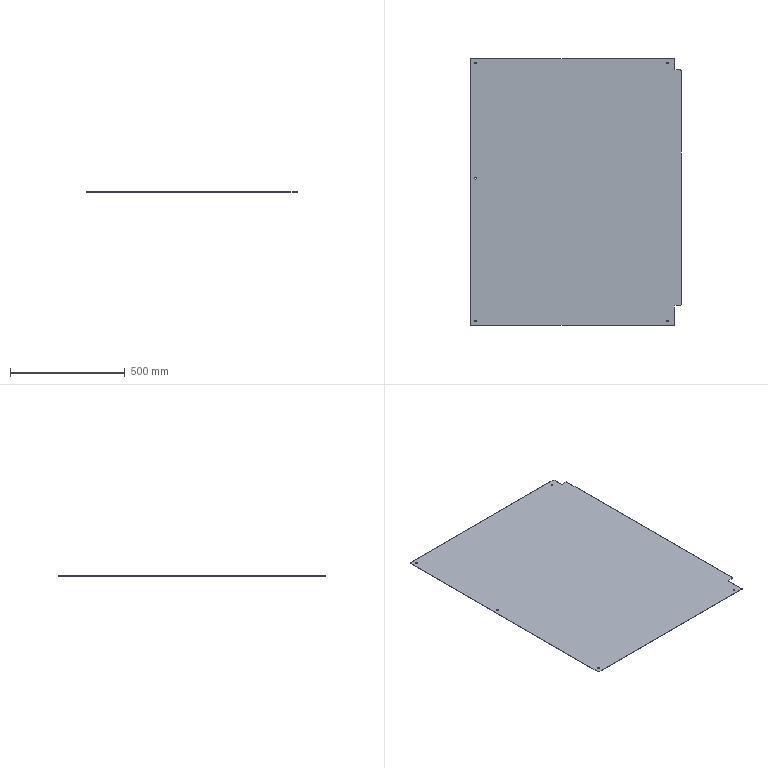Part | SolidWorks | features Fillet 1, FlatPattern 1, HoleWzd 1, ICE 1, SMBaseFlange 1, SheetMetal 1 | 1 solid | 28 faces | box 915 x 1162 x 1.2 mm | volume 1270668 mm3 | cylinder 18 | plane 10 | commonest cylinder face diameters 7 x10 6 x8
STEP:
#1=CARTESIAN_POINT('',(16.5,-20.,0.));
#2=VERTEX_POINT('',#1);
#3=CARTESIAN_POINT('',(23.5,-20.,0.));
#4=VERTEX_POINT('',#3);
#5=CARTESIAN_POINT('',(20.,-20.,0.));
#6=DIRECTION('',(0.,0.,1.));
#7=DIRECTION('',(1.,0.,0.));
#8=AXIS2_PLACEMENT_3D('',#5,#6,#7);
#9=CIRCLE('',#8,3.5);
#10=EDGE_CURVE('',#2,#4,#9,.T.);
#11=ORIENTED_EDGE('',*,*,#10,.F.);
#12=CARTESIAN_POINT('',(16.5,-20.,1.2));
#13=VERTEX_POINT('',#12);
#14=CARTESIAN_POINT('',(16.5,-20.,1.2));
#15=DIRECTION('',(0.,0.,1.));
#16=VECTOR('',#15,1000.);
#17=LINE('',#14,#16);
#18=EDGE_CURVE('',#2,#13,#17,.T.);
#19=ORIENTED_EDGE('',*,*,#18,.T.);
#20=CARTESIAN_POINT('',(23.5,-20.,1.2));
#21=VERTEX_POINT('',#20);
#22=CARTESIAN_POINT('',(20.,-20.,1.2));
#23=DIRECTION('',(0.,0.,1.));
#24=DIRECTION('',(1.,0.,0.));
#25=AXIS2_PLACEMENT_3D('',#22,#23,#24);
#26=CIRCLE('',#25,3.5);
#27=EDGE_CURVE('',#13,#21,#26,.T.);
#28=ORIENTED_EDGE('',*,*,#27,.T.);
#29=CARTESIAN_POINT('',(23.5,-20.,1.2));
#30=DIRECTION('',(0.,0.,1.));
#31=VECTOR('',#30,1000.);
#32=LINE('',#29,#31);
#33=EDGE_CURVE('',#4,#21,#32,.T.);
#34=ORIENTED_EDGE('',*,*,#33,.F.);
#35=EDGE_LOOP('',(#11,#19,#28,#34));
#36=FACE_OUTER_BOUND('',#35,.T.);
#37=CARTESIAN_POINT('',(20.,-20.,1.2));
#38=DIRECTION('',(0.,0.,1.));
#39=DIRECTION('',(1.,0.,0.));
#40=AXIS2_PLACEMENT_3D('',#37,#38,#39);
#41=CYLINDRICAL_SURFACE('',#40,3.5);
#42=ADVANCED_FACE('',(#36),#41,.F.);
#43=CARTESIAN_POINT('',(851.5,-20.,0.));
#44=VERTEX_POINT('',#43);
#45=CARTESIAN_POINT('',(858.5,-20.,0.));
#46=VERTEX_POINT('',#45);
#47=CARTESIAN_POINT('',(855.,-20.,0.));
#48=DIRECTION('',(0.,0.,1.));
#49=DIRECTION('',(1.,0.,0.));
#50=AXIS2_PLACEMENT_3D('',#47,#48,#49);
#51=CIRCLE('',#50,3.5);
#52=EDGE_CURVE('',#44,#46,#51,.T.);
#53=ORIENTED_EDGE('',*,*,#52,.F.);
#54=CARTESIAN_POINT('',(851.5,-20.,1.2));
#55=VERTEX_POINT('',#54);
#56=CARTESIAN_POINT('',(851.5,-20.,1.2));
#57=DIRECTION('',(0.,0.,1.));
#58=VECTOR('',#57,1000.);
#59=LINE('',#56,#58);
#60=EDGE_CURVE('',#44,#55,#59,.T.);
#61=ORIENTED_EDGE('',*,*,#60,.T.);
#62=CARTESIAN_POINT('',(858.5,-20.,1.2));
#63=VERTEX_POINT('',#62);
#64=CARTESIAN_POINT('',(855.,-20.,1.2));
#65=DIRECTION('',(0.,0.,1.));
#66=DIRECTION('',(1.,0.,0.));
#67=AXIS2_PLACEMENT_3D('',#64,#65,#66);
#68=CIRCLE('',#67,3.5);
#69=EDGE_CURVE('',#55,#63,#68,.T.);
#70=ORIENTED_EDGE('',*,*,#69,.T.);
#71=CARTESIAN_POINT('',(858.5,-20.,1.2));
#72=DIRECTION('',(0.,0.,1.));
#73=VECTOR('',#72,1000.);
#74=LINE('',#71,#73);
#75=EDGE_CURVE('',#46,#63,#74,.T.);
#76=ORIENTED_EDGE('',*,*,#75,.F.);
#77=EDGE_LOOP('',(#53,#61,#70,#76));
#78=FACE_OUTER_BOUND('',#77,.T.);
#79=CARTESIAN_POINT('',(855.,-20.,1.2));
#80=DIRECTION('',(0.,0.,1.));
#81=DIRECTION('',(1.,0.,0.));
#82=AXIS2_PLACEMENT_3D('',#79,#80,#81);
#83=CYLINDRICAL_SURFACE('',#82,3.5);
#84=ADVANCED_FACE('',(#78),#83,.F.);
#85=CARTESIAN_POINT('',(16.5,-1142.,0.));
#86=VERTEX_POINT('',#85);
#87=CARTESIAN_POINT('',(23.5,-1142.,0.));
#88=VERTEX_POINT('',#87);
#89=CARTESIAN_POINT('',(20.,-1142.,0.));
#90=DIRECTION('',(0.,0.,1.));
#91=DIRECTION('',(1.,0.,0.));
#92=AXIS2_PLACEMENT_3D('',#89,#90,#91);
#93=CIRCLE('',#92,3.5);
#94=EDGE_CURVE('',#86,#88,#93,.T.);
#95=ORIENTED_EDGE('',*,*,#94,.F.);
#96=CARTESIAN_POINT('',(16.5,-1142.,1.2));
#97=VERTEX_POINT('',#96);
#98=CARTESIAN_POINT('',(16.5,-1142.,1.2));
#99=DIRECTION('',(0.,0.,1.));
#100=VECTOR('',#99,1000.);
#101=LINE('',#98,#100);
#102=EDGE_CURVE('',#86,#97,#101,.T.);
#103=ORIENTED_EDGE('',*,*,#102,.T.);
#104=CARTESIAN_POINT('',(23.5,-1142.,1.2));
#105=VERTEX_POINT('',#104);
#106=CARTESIAN_POINT('',(20.,-1142.,1.2));
#107=DIRECTION('',(0.,0.,1.));
#108=DIRECTION('',(1.,0.,0.));
#109=AXIS2_PLACEMENT_3D('',#106,#107,#108);
#110=CIRCLE('',#109,3.5);
#111=EDGE_CURVE('',#97,#105,#110,.T.);
#112=ORIENTED_EDGE('',*,*,#111,.T.);
#113=CARTESIAN_POINT('',(23.5,-1142.,1.2));
#114=DIRECTION('',(0.,0.,1.));
#115=VECTOR('',#114,1000.);
#116=LINE('',#113,#115);
#117=EDGE_CURVE('',#88,#105,#116,.T.);
#118=ORIENTED_EDGE('',*,*,#117,.F.);
#119=EDGE_LOOP('',(#95,#103,#112,#118));
#120=FACE_OUTER_BOUND('',#119,.T.);
#121=CARTESIAN_POINT('',(20.,-1142.,1.2));
#122=DIRECTION('',(0.,0.,1.));
#123=DIRECTION('',(1.,0.,0.));
#124=AXIS2_PLACEMENT_3D('',#121,#122,#123);
#125=CYLINDRICAL_SURFACE('',#124,3.5);
#126=ADVANCED_FACE('',(#120),#125,.F.);
#127=CARTESIAN_POINT('',(851.5,-1142.,0.));
#128=VERTEX_POINT('',#127);
#129=CARTESIAN_POINT('',(858.5,-1142.,0.));
#130=VERTEX_POINT('',#129);
#131=CARTESIAN_POINT('',(855.,-1142.,0.));
#132=DIRECTION('',(0.,0.,1.));
#133=DIRECTION('',(1.,0.,0.));
#134=AXIS2_PLACEMENT_3D('',#131,#132,#133);
#135=CIRCLE('',#134,3.5);
#136=EDGE_CURVE('',#128,#130,#135,.T.);
#137=ORIENTED_EDGE('',*,*,#136,.F.);
#138=CARTESIAN_POINT('',(851.5,-1142.,1.2));
#139=VERTEX_POINT('',#138);
#140=CARTESIAN_POINT('',(851.5,-1142.,1.2));
#141=DIRECTION('',(0.,0.,1.));
#142=VECTOR('',#141,1000.);
#143=LINE('',#140,#142);
#144=EDGE_CURVE('',#128,#139,#143,.T.);
#145=ORIENTED_EDGE('',*,*,#144,.T.);
#146=CARTESIAN_POINT('',(858.5,-1142.,1.2));
#147=VERTEX_POINT('',#146);
#148=CARTESIAN_POINT('',(855.,-1142.,1.2));
#149=DIRECTION('',(0.,0.,1.));
#150=DIRECTION('',(1.,0.,0.));
#151=AXIS2_PLACEMENT_3D('',#148,#149,#150);
#152=CIRCLE('',#151,3.5);
#153=EDGE_CURVE('',#139,#147,#152,.T.);
#154=ORIENTED_EDGE('',*,*,#153,.T.);
#155=CARTESIAN_POINT('',(858.5,-1142.,1.2));
#156=DIRECTION('',(0.,0.,1.));
#157=VECTOR('',#156,1000.);
#158=LINE('',#155,#157);
#159=EDGE_CURVE('',#130,#147,#158,.T.);
#160=ORIENTED_EDGE('',*,*,#159,.F.);
#161=EDGE_LOOP('',(#137,#145,#154,#160));
#162=FACE_OUTER_BOUND('',#161,.T.);
#163=CARTESIAN_POINT('',(855.,-1142.,1.2));
#164=DIRECTION('',(0.,0.,1.));
#165=DIRECTION('',(1.,0.,0.));
#166=AXIS2_PLACEMENT_3D('',#163,#164,#165);
#167=CYLINDRICAL_SURFACE('',#166,3.5);
#168=ADVANCED_FACE('',(#162),#167,.F.);
#169=CARTESIAN_POINT('',(16.5,-522.,0.));
#170=VERTEX_POINT('',#169);
#171=CARTESIAN_POINT('',(23.5,-522.,0.));
#172=VERTEX_POINT('',#171);
#173=CARTESIAN_POINT('',(20.,-522.,0.));
#174=DIRECTION('',(0.,0.,1.));
#175=DIRECTION('',(1.,0.,0.));
#176=AXIS2_PLACEMENT_3D('',#173,#174,#175);
#177=CIRCLE('',#176,3.5);
#178=EDGE_CURVE('',#170,#172,#177,.T.);
#179=ORIENTED_EDGE('',*,*,#178,.F.);
#180=CARTESIAN_POINT('',(16.5,-522.,1.2));
#181=VERTEX_POINT('',#180);
#182=CARTESIAN_POINT('',(16.5,-522.,1.2));
#183=DIRECTION('',(0.,0.,1.));
#184=VECTOR('',#183,1000.);
#185=LINE('',#182,#184);
#186=EDGE_CURVE('',#170,#181,#185,.T.);
#187=ORIENTED_EDGE('',*,*,#186,.T.);
#188=CARTESIAN_POINT('',(23.5,-522.,1.2));
#189=VERTEX_POINT('',#188);
#190=CARTESIAN_POINT('',(20.,-522.,1.2));
#191=DIRECTION('',(0.,0.,1.));
#192=DIRECTION('',(1.,0.,0.));
#193=AXIS2_PLACEMENT_3D('',#190,#191,#192);
#194=CIRCLE('',#193,3.5);
#195=EDGE_CURVE('',#181,#189,#194,.T.);
#196=ORIENTED_EDGE('',*,*,#195,.T.);
#197=CARTESIAN_POINT('',(23.5,-522.,1.2));
#198=DIRECTION('',(0.,0.,1.));
#199=VECTOR('',#198,1000.);
#200=LINE('',#197,#199);
#201=EDGE_CURVE('',#172,#189,#200,.T.);
#202=ORIENTED_EDGE('',*,*,#201,.F.);
#203=EDGE_LOOP('',(#179,#187,#196,#202));
#204=FACE_OUTER_BOUND('',#203,.T.);
#205=CARTESIAN_POINT('',(20.,-522.,1.2));
#206=DIRECTION('',(0.,0.,1.));
#207=DIRECTION('',(1.,0.,0.));
#208=AXIS2_PLACEMENT_3D('',#205,#206,#207);
#209=CYLINDRICAL_SURFACE('',#208,3.5);
#210=ADVANCED_FACE('',(#204),#209,.F.);
#211=CARTESIAN_POINT('',(0.,-1159.,0.));
#212=VERTEX_POINT('',#211);
#213=CARTESIAN_POINT('',(0.,-3.,0.));
#214=VERTEX_POINT('',#213);
#215=CARTESIAN_POINT('',(0.,0.,0.));
#216=DIRECTION('',(0.,1.,0.));
#217=VECTOR('',#216,1000.);
#218=LINE('',#215,#217);
#219=EDGE_CURVE('',#212,#214,#218,.T.);
#220=ORIENTED_EDGE('',*,*,#219,.F.);
#221=CARTESIAN_POINT('',(0.,-1159.,1.2));
#222=VERTEX_POINT('',#221);
#223=CARTESIAN_POINT('',(0.,-1159.,1.2));
#224=DIRECTION('',(0.,0.,1.));
#225=VECTOR('',#224,1000.);
#226=LINE('',#223,#225);
#227=EDGE_CURVE('',#212,#222,#226,.T.);
#228=ORIENTED_EDGE('',*,*,#227,.T.);
#229=CARTESIAN_POINT('',(0.,-3.,1.2));
#230=VERTEX_POINT('',#229);
#231=CARTESIAN_POINT('',(0.,0.,1.2));
#232=DIRECTION('',(0.,1.,0.));
#233=VECTOR('',#232,1000.);
#234=LINE('',#231,#233);
#235=EDGE_CURVE('',#222,#230,#234,.T.);
#236=ORIENTED_EDGE('',*,*,#235,.T.);
#237=CARTESIAN_POINT('',(0.,-3.,1.2));
#238=DIRECTION('',(0.,0.,-1.));
#239=VECTOR('',#238,1000.);
#240=LINE('',#237,#239);
#241=EDGE_CURVE('',#230,#214,#240,.T.);
#242=ORIENTED_EDGE('',*,*,#241,.T.);
#243=EDGE_LOOP('',(#220,#228,#236,#242));
#244=FACE_OUTER_BOUND('',#243,.T.);
#245=CARTESIAN_POINT('',(0.,0.,1.2));
#246=DIRECTION('',(-1.,0.,0.));
#247=DIRECTION('',(0.,0.,1.));
#248=AXIS2_PLACEMENT_3D('',#245,#246,#247);
#249=PLANE('',#248);
#250=ADVANCED_FACE('',(#244),#249,.T.);
#251=CARTESIAN_POINT('',(882.,-1162.,1.2));
#252=VERTEX_POINT('',#251);
#253=CARTESIAN_POINT('',(3.,-1162.,1.2));
#254=VERTEX_POINT('',#253);
#255=CARTESIAN_POINT('',(0.,-1162.,1.2));
#256=DIRECTION('',(-1.,0.,0.));
#257=VECTOR('',#256,1000.);
#258=LINE('',#255,#257);
#259=EDGE_CURVE('',#252,#254,#258,.T.);
#260=ORIENTED_EDGE('',*,*,#259,.T.);
#261=CARTESIAN_POINT('',(3.,-1162.,0.));
#262=VERTEX_POINT('',#261);
#263=CARTESIAN_POINT('',(3.,-1162.,1.2));
#264=DIRECTION('',(0.,0.,-1.));
#265=VECTOR('',#264,1000.);
#266=LINE('',#263,#265);
#267=EDGE_CURVE('',#254,#262,#266,.T.);
#268=ORIENTED_EDGE('',*,*,#267,.T.);
#269=CARTESIAN_POINT('',(882.,-1162.,0.));
#270=VERTEX_POINT('',#269);
#271=CARTESIAN_POINT('',(0.,-1162.,0.));
#272=DIRECTION('',(-1.,0.,0.));
#273=VECTOR('',#272,1000.);
#274=LINE('',#271,#273);
#275=EDGE_CURVE('',#270,#262,#274,.T.);
#276=ORIENTED_EDGE('',*,*,#275,.F.);
#277=CARTESIAN_POINT('',(882.,-1162.,1.2));
#278=DIRECTION('',(0.,0.,1.));
#279=VECTOR('',#278,1000.);
#280=LINE('',#277,#279);
#281=EDGE_CURVE('',#270,#252,#280,.T.);
#282=ORIENTED_EDGE('',*,*,#281,.T.);
#283=EDGE_LOOP('',(#260,#268,#276,#282));
#284=FACE_OUTER_BOUND('',#283,.T.);
#285=CARTESIAN_POINT('',(0.,-1162.,1.2));
#286=DIRECTION('',(0.,-1.,0.));
#287=DIRECTION('',(0.,0.,-1.));
#288=AXIS2_PLACEMENT_3D('',#285,#286,#287);
#289=PLANE('',#288);
#290=ADVANCED_FACE('',(#284),#289,.T.);
#291=CARTESIAN_POINT('',(915.,-53.,1.2));
#292=VERTEX_POINT('',#291);
#293=CARTESIAN_POINT('',(915.,-1071.,1.2));
#294=VERTEX_POINT('',#293);
#295=CARTESIAN_POINT('',(915.,0.,1.2));
#296=DIRECTION('',(0.,-1.,0.));
#297=VECTOR('',#296,1000.);
#298=LINE('',#295,#297);
#299=EDGE_CURVE('',#292,#294,#298,.T.);
#300=ORIENTED_EDGE('',*,*,#299,.T.);
#301=CARTESIAN_POINT('',(915.,-1071.,0.));
#302=VERTEX_POINT('',#301);
#303=CARTESIAN_POINT('',(915.,-1071.,0.));
#304=DIRECTION('',(0.,0.,-1.));
#305=VECTOR('',#304,1000.);
#306=LINE('',#303,#305);
#307=EDGE_CURVE('',#294,#302,#306,.T.);
#308=ORIENTED_EDGE('',*,*,#307,.T.);
#309=CARTESIAN_POINT('',(915.,-53.,0.));
#310=VERTEX_POINT('',#309);
#311=CARTESIAN_POINT('',(915.,0.,0.));
#312=DIRECTION('',(0.,-1.,0.));
#313=VECTOR('',#312,1000.);
#314=LINE('',#311,#313);
#315=EDGE_CURVE('',#310,#302,#314,.T.);
#316=ORIENTED_EDGE('',*,*,#315,.F.);
#317=CARTESIAN_POINT('',(915.,-53.,1.2));
#318=DIRECTION('',(0.,0.,1.));
#319=VECTOR('',#318,1000.);
#320=LINE('',#317,#319);
#321=EDGE_CURVE('',#310,#292,#320,.T.);
#322=ORIENTED_EDGE('',*,*,#321,.T.);
#323=EDGE_LOOP('',(#300,#308,#316,#322));
#324=FACE_OUTER_BOUND('',#323,.T.);
#325=CARTESIAN_POINT('',(915.,0.,1.2));
#326=DIRECTION('',(1.,0.,0.));
#327=DIRECTION('',(0.,0.,-1.));
#328=AXIS2_PLACEMENT_3D('',#325,#326,#327);
#329=PLANE('',#328);
#330=ADVANCED_FACE('',(#324),#329,.T.);
#331=CARTESIAN_POINT('',(3.,0.,1.2));
#332=VERTEX_POINT('',#331);
#333=CARTESIAN_POINT('',(882.,0.,1.2));
#334=VERTEX_POINT('',#333);
#335=CARTESIAN_POINT('',(0.,0.,1.2));
#336=DIRECTION('',(1.,0.,0.));
#337=VECTOR('',#336,1000.);
#338=LINE('',#335,#337);
#339=EDGE_CURVE('',#332,#334,#338,.T.);
#340=ORIENTED_EDGE('',*,*,#339,.T.);
#341=CARTESIAN_POINT('',(882.,0.,0.));
#342=VERTEX_POINT('',#341);
#343=CARTESIAN_POINT('',(882.,0.,0.));
#344=DIRECTION('',(0.,0.,-1.));
#345=VECTOR('',#344,1000.);
#346=LINE('',#343,#345);
#347=EDGE_CURVE('',#334,#342,#346,.T.);
#348=ORIENTED_EDGE('',*,*,#347,.T.);
#349=CARTESIAN_POINT('',(3.,0.,0.));
#350=VERTEX_POINT('',#349);
#351=CARTESIAN_POINT('',(0.,0.,0.));
#352=DIRECTION('',(1.,0.,0.));
#353=VECTOR('',#352,1000.);
#354=LINE('',#351,#353);
#355=EDGE_CURVE('',#350,#342,#354,.T.);
#356=ORIENTED_EDGE('',*,*,#355,.F.);
#357=CARTESIAN_POINT('',(3.,0.,1.2));
#358=DIRECTION('',(0.,0.,1.));
#359=VECTOR('',#358,1000.);
#360=LINE('',#357,#359);
#361=EDGE_CURVE('',#350,#332,#360,.T.);
#362=ORIENTED_EDGE('',*,*,#361,.T.);
#363=EDGE_LOOP('',(#340,#348,#356,#362));
#364=FACE_OUTER_BOUND('',#363,.T.);
#365=CARTESIAN_POINT('',(0.,0.,1.2));
#366=DIRECTION('',(0.,1.,0.));
#367=DIRECTION('',(0.,0.,1.));
#368=AXIS2_PLACEMENT_3D('',#365,#366,#367);
#369=PLANE('',#368);
#370=ADVANCED_FACE('',(#364),#369,.T.);
#371=CARTESIAN_POINT('',(20.,-20.,1.2));
#372=DIRECTION('',(0.,0.,1.));
#373=DIRECTION('',(1.,0.,0.));
#374=AXIS2_PLACEMENT_3D('',#371,#372,#373);
#375=CIRCLE('',#374,3.5);
#376=EDGE_CURVE('',#21,#13,#375,.T.);
#377=ORIENTED_EDGE('',*,*,#376,.F.);
#378=ORIENTED_EDGE('',*,*,#27,.F.);
#379=EDGE_LOOP('',(#377,#378));
#380=FACE_BOUND('',#379,.T.);
#381=CARTESIAN_POINT('',(855.,-20.,1.2));
#382=DIRECTION('',(0.,0.,1.));
#383=DIRECTION('',(1.,0.,0.));
#384=AXIS2_PLACEMENT_3D('',#381,#382,#383);
#385=CIRCLE('',#384,3.5);
#386=EDGE_CURVE('',#63,#55,#385,.T.);
#387=ORIENTED_EDGE('',*,*,#386,.F.);
#388=ORIENTED_EDGE('',*,*,#69,.F.);
#389=EDGE_LOOP('',(#387,#388));
#390=FACE_BOUND('',#389,.T.);
#391=CARTESIAN_POINT('',(20.,-1142.,1.2));
#392=DIRECTION('',(0.,0.,1.));
#393=DIRECTION('',(1.,0.,0.));
#394=AXIS2_PLACEMENT_3D('',#391,#392,#393);
#395=CIRCLE('',#394,3.5);
#396=EDGE_CURVE('',#105,#97,#395,.T.);
#397=ORIENTED_EDGE('',*,*,#396,.F.);
#398=ORIENTED_EDGE('',*,*,#111,.F.);
#399=EDGE_LOOP('',(#397,#398));
#400=FACE_BOUND('',#399,.T.);
#401=CARTESIAN_POINT('',(855.,-1142.,1.2));
#402=DIRECTION('',(0.,0.,1.));
#403=DIRECTION('',(1.,0.,0.));
#404=AXIS2_PLACEMENT_3D('',#401,#402,#403);
#405=CIRCLE('',#404,3.5);
#406=EDGE_CURVE('',#147,#139,#405,.T.);
#407=ORIENTED_EDGE('',*,*,#406,.F.);
#408=ORIENTED_EDGE('',*,*,#153,.F.);
#409=EDGE_LOOP('',(#407,#408));
#410=FACE_BOUND('',#409,.T.);
#411=CARTESIAN_POINT('',(20.,-522.,1.2));
#412=DIRECTION('',(0.,0.,1.));
#413=DIRECTION('',(1.,0.,0.));
#414=AXIS2_PLACEMENT_3D('',#411,#412,#413);
#415=CIRCLE('',#414,3.5);
#416=EDGE_CURVE('',#189,#181,#415,.T.);
#417=ORIENTED_EDGE('',*,*,#416,.F.);
#418=ORIENTED_EDGE('',*,*,#195,.F.);
#419=EDGE_LOOP('',(#417,#418));
#420=FACE_BOUND('',#419,.T.);
#421=ORIENTED_EDGE('',*,*,#235,.F.);
#422=CARTESIAN_POINT('',(3.,-1159.,1.2));
#423=DIRECTION('',(0.,0.,1.));
#424=DIRECTION('',(1.,0.,0.));
#425=AXIS2_PLACEMENT_3D('',#422,#423,#424);
#426=CIRCLE('',#425,3.);
#427=EDGE_CURVE('',#222,#254,#426,.T.);
#428=ORIENTED_EDGE('',*,*,#427,.T.);
#429=ORIENTED_EDGE('',*,*,#259,.F.);
#430=CARTESIAN_POINT('',(885.,-1159.,1.2));
#431=VERTEX_POINT('',#430);
#432=CARTESIAN_POINT('',(882.,-1159.,1.2));
#433=DIRECTION('',(0.,0.,1.));
#434=DIRECTION('',(1.,0.,0.));
#435=AXIS2_PLACEMENT_3D('',#432,#433,#434);
#436=CIRCLE('',#435,3.);
#437=EDGE_CURVE('',#252,#431,#436,.T.);
#438=ORIENTED_EDGE('',*,*,#437,.T.);
#439=CARTESIAN_POINT('',(885.,-1077.,1.2));
#440=VERTEX_POINT('',#439);
#441=CARTESIAN_POINT('',(885.,-1162.,1.2));
#442=DIRECTION('',(0.,-1.,0.));
#443=VECTOR('',#442,1000.);
#444=LINE('',#441,#443);
#445=EDGE_CURVE('',#440,#431,#444,.T.);
#446=ORIENTED_EDGE('',*,*,#445,.F.);
#447=CARTESIAN_POINT('',(888.,-1074.,1.2));
#448=VERTEX_POINT('',#447);
#449=CARTESIAN_POINT('',(888.,-1077.,1.2));
#450=DIRECTION('',(0.,0.,-1.));
#451=DIRECTION('',(1.,0.,0.));
#452=AXIS2_PLACEMENT_3D('',#449,#450,#451);
#453=CIRCLE('',#452,3.);
#454=EDGE_CURVE('',#440,#448,#453,.T.);
#455=ORIENTED_EDGE('',*,*,#454,.T.);
#456=CARTESIAN_POINT('',(912.,-1074.,1.2));
#457=VERTEX_POINT('',#456);
#458=CARTESIAN_POINT('',(915.,-1074.,1.2));
#459=DIRECTION('',(-1.,0.,0.));
#460=VECTOR('',#459,1000.);
#461=LINE('',#458,#460);
#462=EDGE_CURVE('',#457,#448,#461,.T.);
#463=ORIENTED_EDGE('',*,*,#462,.F.);
#464=CARTESIAN_POINT('',(912.,-1071.,1.2));
#465=DIRECTION('',(0.,0.,1.));
#466=DIRECTION('',(1.,0.,0.));
#467=AXIS2_PLACEMENT_3D('',#464,#465,#466);
#468=CIRCLE('',#467,3.);
#469=EDGE_CURVE('',#457,#294,#468,.T.);
#470=ORIENTED_EDGE('',*,*,#469,.T.);
#471=ORIENTED_EDGE('',*,*,#299,.F.);
#472=CARTESIAN_POINT('',(912.,-50.,1.2));
#473=VERTEX_POINT('',#472);
#474=CARTESIAN_POINT('',(912.,-53.,1.2));
#475=DIRECTION('',(0.,0.,1.));
#476=DIRECTION('',(1.,0.,0.));
#477=AXIS2_PLACEMENT_3D('',#474,#475,#476);
#478=CIRCLE('',#477,3.);
#479=EDGE_CURVE('',#292,#473,#478,.T.);
#480=ORIENTED_EDGE('',*,*,#479,.T.);
#481=CARTESIAN_POINT('',(888.,-50.,1.2));
#482=VERTEX_POINT('',#481);
#483=CARTESIAN_POINT('',(915.,-50.,1.2));
#484=DIRECTION('',(1.,0.,0.));
#485=VECTOR('',#484,1000.);
#486=LINE('',#483,#485);
#487=EDGE_CURVE('',#482,#473,#486,.T.);
#488=ORIENTED_EDGE('',*,*,#487,.F.);
#489=CARTESIAN_POINT('',(885.,-47.,1.2));
#490=VERTEX_POINT('',#489);
#491=CARTESIAN_POINT('',(888.,-47.,1.2));
#492=DIRECTION('',(0.,0.,-1.));
#493=DIRECTION('',(1.,0.,0.));
#494=AXIS2_PLACEMENT_3D('',#491,#492,#493);
#495=CIRCLE('',#494,3.);
#496=EDGE_CURVE('',#482,#490,#495,.T.);
#497=ORIENTED_EDGE('',*,*,#496,.T.);
#498=CARTESIAN_POINT('',(885.,-3.,1.2));
#499=VERTEX_POINT('',#498);
#500=CARTESIAN_POINT('',(885.,0.,1.2));
#501=DIRECTION('',(0.,-1.,0.));
#502=VECTOR('',#501,1000.);
#503=LINE('',#500,#502);
#504=EDGE_CURVE('',#499,#490,#503,.T.);
#505=ORIENTED_EDGE('',*,*,#504,.F.);
#506=CARTESIAN_POINT('',(882.,-3.,1.2));
#507=DIRECTION('',(0.,0.,1.));
#508=DIRECTION('',(1.,0.,0.));
#509=AXIS2_PLACEMENT_3D('',#506,#507,#508);
#510=CIRCLE('',#509,3.);
#511=EDGE_CURVE('',#499,#334,#510,.T.);
#512=ORIENTED_EDGE('',*,*,#511,.T.);
#513=ORIENTED_EDGE('',*,*,#339,.F.);
#514=CARTESIAN_POINT('',(3.,-3.,1.2));
#515=DIRECTION('',(0.,0.,1.));
#516=DIRECTION('',(1.,0.,0.));
#517=AXIS2_PLACEMENT_3D('',#514,#515,#516);
#518=CIRCLE('',#517,3.);
#519=EDGE_CURVE('',#332,#230,#518,.T.);
#520=ORIENTED_EDGE('',*,*,#519,.T.);
#521=EDGE_LOOP('',(#421,#428,#429,#438,#446,#455,#463,#470,#471,#480,#488,#497,#505,#512,#513,#520));
#522=FACE_OUTER_BOUND('',#521,.T.);
#523=CARTESIAN_POINT('',(0.,0.,1.2));
#524=DIRECTION('',(0.,0.,1.));
#525=DIRECTION('',(1.,0.,0.));
#526=AXIS2_PLACEMENT_3D('',#523,#524,#525);
#527=PLANE('',#526);
#528=ADVANCED_FACE('',(#380,#390,#400,#410,#420,#522),#527,.T.);
#529=CARTESIAN_POINT('',(20.,-20.,0.));
#530=DIRECTION('',(0.,0.,1.));
#531=DIRECTION('',(1.,0.,0.));
#532=AXIS2_PLACEMENT_3D('',#529,#530,#531);
#533=CIRCLE('',#532,3.5);
#534=EDGE_CURVE('',#4,#2,#533,.T.);
#535=ORIENTED_EDGE('',*,*,#534,.T.);
#536=ORIENTED_EDGE('',*,*,#10,.T.);
#537=EDGE_LOOP('',(#535,#536));
#538=FACE_BOUND('',#537,.T.);
#539=CARTESIAN_POINT('',(855.,-20.,0.));
#540=DIRECTION('',(0.,0.,1.));
#541=DIRECTION('',(1.,0.,0.));
#542=AXIS2_PLACEMENT_3D('',#539,#540,#541);
#543=CIRCLE('',#542,3.5);
#544=EDGE_CURVE('',#46,#44,#543,.T.);
#545=ORIENTED_EDGE('',*,*,#544,.T.);
#546=ORIENTED_EDGE('',*,*,#52,.T.);
#547=EDGE_LOOP('',(#545,#546));
#548=FACE_BOUND('',#547,.T.);
#549=CARTESIAN_POINT('',(20.,-1142.,0.));
#550=DIRECTION('',(0.,0.,1.));
#551=DIRECTION('',(1.,0.,0.));
#552=AXIS2_PLACEMENT_3D('',#549,#550,#551);
#553=CIRCLE('',#552,3.5);
#554=EDGE_CURVE('',#88,#86,#553,.T.);
#555=ORIENTED_EDGE('',*,*,#554,.T.);
#556=ORIENTED_EDGE('',*,*,#94,.T.);
#557=EDGE_LOOP('',(#555,#556));
#558=FACE_BOUND('',#557,.T.);
#559=CARTESIAN_POINT('',(855.,-1142.,0.));
#560=DIRECTION('',(0.,0.,1.));
#561=DIRECTION('',(1.,0.,0.));
#562=AXIS2_PLACEMENT_3D('',#559,#560,#561);
#563=CIRCLE('',#562,3.5);
#564=EDGE_CURVE('',#130,#128,#563,.T.);
#565=ORIENTED_EDGE('',*,*,#564,.T.);
#566=ORIENTED_EDGE('',*,*,#136,.T.);
#567=EDGE_LOOP('',(#565,#566));
#568=FACE_BOUND('',#567,.T.);
#569=CARTESIAN_POINT('',(20.,-522.,0.));
#570=DIRECTION('',(0.,0.,1.));
#571=DIRECTION('',(1.,0.,0.));
#572=AXIS2_PLACEMENT_3D('',#569,#570,#571);
#573=CIRCLE('',#572,3.5);
#574=EDGE_CURVE('',#172,#170,#573,.T.);
#575=ORIENTED_EDGE('',*,*,#574,.T.);
#576=ORIENTED_EDGE('',*,*,#178,.T.);
#577=EDGE_LOOP('',(#575,#576));
#578=FACE_BOUND('',#577,.T.);
#579=ORIENTED_EDGE('',*,*,#275,.T.);
#580=CARTESIAN_POINT('',(3.,-1159.,0.));
#581=DIRECTION('',(0.,0.,-1.));
#582=DIRECTION('',(1.,0.,0.));
#583=AXIS2_PLACEMENT_3D('',#580,#581,#582);
#584=CIRCLE('',#583,3.);
#585=EDGE_CURVE('',#262,#212,#584,.T.);
#586=ORIENTED_EDGE('',*,*,#585,.T.);
#587=ORIENTED_EDGE('',*,*,#219,.T.);
#588=CARTESIAN_POINT('',(3.,-3.,0.));
#589=DIRECTION('',(0.,0.,-1.));
#590=DIRECTION('',(1.,0.,0.));
#591=AXIS2_PLACEMENT_3D('',#588,#589,#590);
#592=CIRCLE('',#591,3.);
#593=EDGE_CURVE('',#214,#350,#592,.T.);
#594=ORIENTED_EDGE('',*,*,#593,.T.);
#595=ORIENTED_EDGE('',*,*,#355,.T.);
#596=CARTESIAN_POINT('',(885.,-3.,0.));
#597=VERTEX_POINT('',#596);
#598=CARTESIAN_POINT('',(882.,-3.,0.));
#599=DIRECTION('',(0.,0.,-1.));
#600=DIRECTION('',(1.,0.,0.));
#601=AXIS2_PLACEMENT_3D('',#598,#599,#600);
#602=CIRCLE('',#601,3.);
#603=EDGE_CURVE('',#342,#597,#602,.T.);
#604=ORIENTED_EDGE('',*,*,#603,.T.);
#605=CARTESIAN_POINT('',(885.,-47.,0.));
#606=VERTEX_POINT('',#605);
#607=CARTESIAN_POINT('',(885.,0.,0.));
#608=DIRECTION('',(0.,-1.,0.));
#609=VECTOR('',#608,1000.);
#610=LINE('',#607,#609);
#611=EDGE_CURVE('',#597,#606,#610,.T.);
#612=ORIENTED_EDGE('',*,*,#611,.T.);
#613=CARTESIAN_POINT('',(888.,-50.,0.));
#614=VERTEX_POINT('',#613);
#615=CARTESIAN_POINT('',(888.,-47.,0.));
#616=DIRECTION('',(0.,0.,1.));
#617=DIRECTION('',(1.,0.,0.));
#618=AXIS2_PLACEMENT_3D('',#615,#616,#617);
#619=CIRCLE('',#618,3.);
#620=EDGE_CURVE('',#606,#614,#619,.T.);
#621=ORIENTED_EDGE('',*,*,#620,.T.);
#622=CARTESIAN_POINT('',(912.,-50.,0.));
#623=VERTEX_POINT('',#622);
#624=CARTESIAN_POINT('',(0.,-50.,0.));
#625=DIRECTION('',(1.,0.,0.));
#626=VECTOR('',#625,1000.);
#627=LINE('',#624,#626);
#628=EDGE_CURVE('',#614,#623,#627,.T.);
#629=ORIENTED_EDGE('',*,*,#628,.T.);
#630=CARTESIAN_POINT('',(912.,-53.,0.));
#631=DIRECTION('',(0.,0.,-1.));
#632=DIRECTION('',(1.,0.,0.));
#633=AXIS2_PLACEMENT_3D('',#630,#631,#632);
#634=CIRCLE('',#633,3.);
#635=EDGE_CURVE('',#623,#310,#634,.T.);
#636=ORIENTED_EDGE('',*,*,#635,.T.);
#637=ORIENTED_EDGE('',*,*,#315,.T.);
#638=CARTESIAN_POINT('',(912.,-1074.,0.));
#639=VERTEX_POINT('',#638);
#640=CARTESIAN_POINT('',(912.,-1071.,0.));
#641=DIRECTION('',(0.,0.,-1.));
#642=DIRECTION('',(1.,0.,0.));
#643=AXIS2_PLACEMENT_3D('',#640,#641,#642);
#644=CIRCLE('',#643,3.);
#645=EDGE_CURVE('',#302,#639,#644,.T.);
#646=ORIENTED_EDGE('',*,*,#645,.T.);
#647=CARTESIAN_POINT('',(888.,-1074.,0.));
#648=VERTEX_POINT('',#647);
#649=CARTESIAN_POINT('',(0.,-1074.,0.));
#650=DIRECTION('',(-1.,0.,0.));
#651=VECTOR('',#650,1000.);
#652=LINE('',#649,#651);
#653=EDGE_CURVE('',#639,#648,#652,.T.);
#654=ORIENTED_EDGE('',*,*,#653,.T.);
#655=CARTESIAN_POINT('',(885.,-1077.,0.));
#656=VERTEX_POINT('',#655);
#657=CARTESIAN_POINT('',(888.,-1077.,0.));
#658=DIRECTION('',(0.,0.,1.));
#659=DIRECTION('',(1.,0.,0.));
#660=AXIS2_PLACEMENT_3D('',#657,#658,#659);
#661=CIRCLE('',#660,3.);
#662=EDGE_CURVE('',#648,#656,#661,.T.);
#663=ORIENTED_EDGE('',*,*,#662,.T.);
#664=CARTESIAN_POINT('',(885.,-1159.,0.));
#665=VERTEX_POINT('',#664);
#666=CARTESIAN_POINT('',(885.,0.,0.));
#667=DIRECTION('',(0.,-1.,0.));
#668=VECTOR('',#667,1000.);
#669=LINE('',#666,#668);
#670=EDGE_CURVE('',#656,#665,#669,.T.);
#671=ORIENTED_EDGE('',*,*,#670,.T.);
#672=CARTESIAN_POINT('',(882.,-1159.,0.));
#673=DIRECTION('',(0.,0.,-1.));
#674=DIRECTION('',(1.,0.,0.));
#675=AXIS2_PLACEMENT_3D('',#672,#673,#674);
#676=CIRCLE('',#675,3.);
#677=EDGE_CURVE('',#665,#270,#676,.T.);
#678=ORIENTED_EDGE('',*,*,#677,.T.);
#679=EDGE_LOOP('',(#579,#586,#587,#594,#595,#604,#612,#621,#629,#636,#637,#646,#654,#663,#671,#678));
#680=FACE_OUTER_BOUND('',#679,.T.);
#681=CARTESIAN_POINT('',(0.,0.,0.));
#682=DIRECTION('',(0.,0.,1.));
#683=DIRECTION('',(1.,0.,0.));
#684=AXIS2_PLACEMENT_3D('',#681,#682,#683);
#685=PLANE('',#684);
#686=ADVANCED_FACE('',(#538,#548,#558,#568,#578,#680),#685,.F.);
#687=ORIENTED_EDGE('',*,*,#445,.T.);
#688=CARTESIAN_POINT('',(885.,-1159.,0.));
#689=DIRECTION('',(0.,0.,-1.));
#690=VECTOR('',#689,1000.);
#691=LINE('',#688,#690);
#692=EDGE_CURVE('',#431,#665,#691,.T.);
#693=ORIENTED_EDGE('',*,*,#692,.T.);
#694=ORIENTED_EDGE('',*,*,#670,.F.);
#695=CARTESIAN_POINT('',(885.,-1077.,1.2));
#696=DIRECTION('',(0.,0.,1.));
#697=VECTOR('',#696,1000.);
#698=LINE('',#695,#697);
#699=EDGE_CURVE('',#656,#440,#698,.T.);
#700=ORIENTED_EDGE('',*,*,#699,.T.);
#701=EDGE_LOOP('',(#687,#693,#694,#700));
#702=FACE_OUTER_BOUND('',#701,.T.);
#703=CARTESIAN_POINT('',(885.,-1162.,-8.8));
#704=DIRECTION('',(-1.,0.,0.));
#705=DIRECTION('',(0.,0.,1.));
#706=AXIS2_PLACEMENT_3D('',#703,#704,#705);
#707=PLANE('',#706);
#708=ADVANCED_FACE('',(#702),#707,.F.);
#709=ORIENTED_EDGE('',*,*,#462,.T.);
#710=CARTESIAN_POINT('',(888.,-1074.,0.));
#711=DIRECTION('',(0.,0.,-1.));
#712=VECTOR('',#711,1000.);
#713=LINE('',#710,#712);
#714=EDGE_CURVE('',#448,#648,#713,.T.);
#715=ORIENTED_EDGE('',*,*,#714,.T.);
#716=ORIENTED_EDGE('',*,*,#653,.F.);
#717=CARTESIAN_POINT('',(912.,-1074.,1.2));
#718=DIRECTION('',(0.,0.,1.));
#719=VECTOR('',#718,1000.);
#720=LINE('',#717,#719);
#721=EDGE_CURVE('',#639,#457,#720,.T.);
#722=ORIENTED_EDGE('',*,*,#721,.T.);
#723=EDGE_LOOP('',(#709,#715,#716,#722));
#724=FACE_OUTER_BOUND('',#723,.T.);
#725=CARTESIAN_POINT('',(915.,-1074.,-8.8));
#726=DIRECTION('',(0.,1.,0.));
#727=DIRECTION('',(0.,0.,1.));
#728=AXIS2_PLACEMENT_3D('',#725,#726,#727);
#729=PLANE('',#728);
#730=ADVANCED_FACE('',(#724),#729,.F.);
#731=ORIENTED_EDGE('',*,*,#487,.T.);
#732=CARTESIAN_POINT('',(912.,-50.,0.));
#733=DIRECTION('',(0.,0.,-1.));
#734=VECTOR('',#733,1000.);
#735=LINE('',#732,#734);
#736=EDGE_CURVE('',#473,#623,#735,.T.);
#737=ORIENTED_EDGE('',*,*,#736,.T.);
#738=ORIENTED_EDGE('',*,*,#628,.F.);
#739=CARTESIAN_POINT('',(888.,-50.,1.2));
#740=DIRECTION('',(0.,0.,1.));
#741=VECTOR('',#740,1000.);
#742=LINE('',#739,#741);
#743=EDGE_CURVE('',#614,#482,#742,.T.);
#744=ORIENTED_EDGE('',*,*,#743,.T.);
#745=EDGE_LOOP('',(#731,#737,#738,#744));
#746=FACE_OUTER_BOUND('',#745,.T.);
#747=CARTESIAN_POINT('',(915.,-50.,-8.8));
#748=DIRECTION('',(0.,-1.,0.));
#749=DIRECTION('',(1.,0.,0.));
#750=AXIS2_PLACEMENT_3D('',#747,#748,#749);
#751=PLANE('',#750);
#752=ADVANCED_FACE('',(#746),#751,.F.);
#753=ORIENTED_EDGE('',*,*,#504,.T.);
#754=CARTESIAN_POINT('',(885.,-47.,0.));
#755=DIRECTION('',(0.,0.,-1.));
#756=VECTOR('',#755,1000.);
#757=LINE('',#754,#756);
#758=EDGE_CURVE('',#490,#606,#757,.T.);
#759=ORIENTED_EDGE('',*,*,#758,.T.);
#760=ORIENTED_EDGE('',*,*,#611,.F.);
#761=CARTESIAN_POINT('',(885.,-3.,1.2));
#762=DIRECTION('',(0.,0.,1.));
#763=VECTOR('',#762,1000.);
#764=LINE('',#761,#763);
#765=EDGE_CURVE('',#597,#499,#764,.T.);
#766=ORIENTED_EDGE('',*,*,#765,.T.);
#767=EDGE_LOOP('',(#753,#759,#760,#766));
#768=FACE_OUTER_BOUND('',#767,.T.);
#769=CARTESIAN_POINT('',(885.,0.,-8.8));
#770=DIRECTION('',(-1.,0.,0.));
#771=DIRECTION('',(0.,0.,1.));
#772=AXIS2_PLACEMENT_3D('',#769,#770,#771);
#773=PLANE('',#772);
#774=ADVANCED_FACE('',(#768),#773,.F.);
#775=ORIENTED_EDGE('',*,*,#186,.F.);
#776=ORIENTED_EDGE('',*,*,#574,.F.);
#777=ORIENTED_EDGE('',*,*,#201,.T.);
#778=ORIENTED_EDGE('',*,*,#416,.T.);
#779=EDGE_LOOP('',(#775,#776,#777,#778));
#780=FACE_OUTER_BOUND('',#779,.T.);
#781=CARTESIAN_POINT('',(20.,-522.,1.2));
#782=DIRECTION('',(0.,0.,1.));
#783=DIRECTION('',(1.,0.,0.));
#784=AXIS2_PLACEMENT_3D('',#781,#782,#783);
#785=CYLINDRICAL_SURFACE('',#784,3.5);
#786=ADVANCED_FACE('',(#780),#785,.F.);
#787=ORIENTED_EDGE('',*,*,#144,.F.);
#788=ORIENTED_EDGE('',*,*,#564,.F.);
#789=ORIENTED_EDGE('',*,*,#159,.T.);
#790=ORIENTED_EDGE('',*,*,#406,.T.);
#791=EDGE_LOOP('',(#787,#788,#789,#790));
#792=FACE_OUTER_BOUND('',#791,.T.);
#793=CARTESIAN_POINT('',(855.,-1142.,1.2));
#794=DIRECTION('',(0.,0.,1.));
#795=DIRECTION('',(1.,0.,0.));
#796=AXIS2_PLACEMENT_3D('',#793,#794,#795);
#797=CYLINDRICAL_SURFACE('',#796,3.5);
#798=ADVANCED_FACE('',(#792),#797,.F.);
#799=ORIENTED_EDGE('',*,*,#102,.F.);
#800=ORIENTED_EDGE('',*,*,#554,.F.);
#801=ORIENTED_EDGE('',*,*,#117,.T.);
#802=ORIENTED_EDGE('',*,*,#396,.T.);
#803=EDGE_LOOP('',(#799,#800,#801,#802));
#804=FACE_OUTER_BOUND('',#803,.T.);
#805=CARTESIAN_POINT('',(20.,-1142.,1.2));
#806=DIRECTION('',(0.,0.,1.));
#807=DIRECTION('',(1.,0.,0.));
#808=AXIS2_PLACEMENT_3D('',#805,#806,#807);
#809=CYLINDRICAL_SURFACE('',#808,3.5);
#810=ADVANCED_FACE('',(#804),#809,.F.);
#811=ORIENTED_EDGE('',*,*,#60,.F.);
#812=ORIENTED_EDGE('',*,*,#544,.F.);
#813=ORIENTED_EDGE('',*,*,#75,.T.);
#814=ORIENTED_EDGE('',*,*,#386,.T.);
#815=EDGE_LOOP('',(#811,#812,#813,#814));
#816=FACE_OUTER_BOUND('',#815,.T.);
#817=CARTESIAN_POINT('',(855.,-20.,1.2));
#818=DIRECTION('',(0.,0.,1.));
#819=DIRECTION('',(1.,0.,0.));
#820=AXIS2_PLACEMENT_3D('',#817,#818,#819);
#821=CYLINDRICAL_SURFACE('',#820,3.5);
#822=ADVANCED_FACE('',(#816),#821,.F.);
#823=ORIENTED_EDGE('',*,*,#18,.F.);
#824=ORIENTED_EDGE('',*,*,#534,.F.);
#825=ORIENTED_EDGE('',*,*,#33,.T.);
#826=ORIENTED_EDGE('',*,*,#376,.T.);
#827=EDGE_LOOP('',(#823,#824,#825,#826));
#828=FACE_OUTER_BOUND('',#827,.T.);
#829=CARTESIAN_POINT('',(20.,-20.,1.2));
#830=DIRECTION('',(0.,0.,1.));
#831=DIRECTION('',(1.,0.,0.));
#832=AXIS2_PLACEMENT_3D('',#829,#830,#831);
#833=CYLINDRICAL_SURFACE('',#832,3.5);
#834=ADVANCED_FACE('',(#828),#833,.F.);
#835=ORIENTED_EDGE('',*,*,#427,.F.);
#836=ORIENTED_EDGE('',*,*,#227,.F.);
#837=ORIENTED_EDGE('',*,*,#585,.F.);
#838=ORIENTED_EDGE('',*,*,#267,.F.);
#839=EDGE_LOOP('',(#835,#836,#837,#838));
#840=FACE_OUTER_BOUND('',#839,.T.);
#841=CARTESIAN_POINT('',(3.,-1159.,1.2));
#842=DIRECTION('',(0.,0.,-1.));
#843=DIRECTION('',(-1.,0.,0.));
#844=AXIS2_PLACEMENT_3D('',#841,#842,#843);
#845=CYLINDRICAL_SURFACE('',#844,3.);
#846=ADVANCED_FACE('',(#840),#845,.T.);
#847=ORIENTED_EDGE('',*,*,#677,.F.);
#848=ORIENTED_EDGE('',*,*,#692,.F.);
#849=ORIENTED_EDGE('',*,*,#437,.F.);
#850=ORIENTED_EDGE('',*,*,#281,.F.);
#851=EDGE_LOOP('',(#847,#848,#849,#850));
#852=FACE_OUTER_BOUND('',#851,.T.);
#853=CARTESIAN_POINT('',(882.,-1159.,1.2));
#854=DIRECTION('',(0.,0.,-1.));
#855=DIRECTION('',(-1.,0.,0.));
#856=AXIS2_PLACEMENT_3D('',#853,#854,#855);
#857=CYLINDRICAL_SURFACE('',#856,3.);
#858=ADVANCED_FACE('',(#852),#857,.T.);
#859=ORIENTED_EDGE('',*,*,#662,.F.);
#860=ORIENTED_EDGE('',*,*,#714,.F.);
#861=ORIENTED_EDGE('',*,*,#454,.F.);
#862=ORIENTED_EDGE('',*,*,#699,.F.);
#863=EDGE_LOOP('',(#859,#860,#861,#862));
#864=FACE_OUTER_BOUND('',#863,.T.);
#865=CARTESIAN_POINT('',(888.,-1077.,-8.8));
#866=DIRECTION('',(0.,0.,-1.));
#867=DIRECTION('',(-1.,0.,0.));
#868=AXIS2_PLACEMENT_3D('',#865,#866,#867);
#869=CYLINDRICAL_SURFACE('',#868,3.);
#870=ADVANCED_FACE('',(#864),#869,.F.);
#871=ORIENTED_EDGE('',*,*,#645,.F.);
#872=ORIENTED_EDGE('',*,*,#307,.F.);
#873=ORIENTED_EDGE('',*,*,#469,.F.);
#874=ORIENTED_EDGE('',*,*,#721,.F.);
#875=EDGE_LOOP('',(#871,#872,#873,#874));
#876=FACE_OUTER_BOUND('',#875,.T.);
#877=CARTESIAN_POINT('',(912.,-1071.,-8.8));
#878=DIRECTION('',(0.,0.,-1.));
#879=DIRECTION('',(-1.,0.,0.));
#880=AXIS2_PLACEMENT_3D('',#877,#878,#879);
#881=CYLINDRICAL_SURFACE('',#880,3.);
#882=ADVANCED_FACE('',(#876),#881,.T.);
#883=ORIENTED_EDGE('',*,*,#635,.F.);
#884=ORIENTED_EDGE('',*,*,#736,.F.);
#885=ORIENTED_EDGE('',*,*,#479,.F.);
#886=ORIENTED_EDGE('',*,*,#321,.F.);
#887=EDGE_LOOP('',(#883,#884,#885,#886));
#888=FACE_OUTER_BOUND('',#887,.T.);
#889=CARTESIAN_POINT('',(912.,-53.,1.2));
#890=DIRECTION('',(0.,0.,-1.));
#891=DIRECTION('',(-1.,0.,0.));
#892=AXIS2_PLACEMENT_3D('',#889,#890,#891);
#893=CYLINDRICAL_SURFACE('',#892,3.);
#894=ADVANCED_FACE('',(#888),#893,.T.);
#895=ORIENTED_EDGE('',*,*,#620,.F.);
#896=ORIENTED_EDGE('',*,*,#758,.F.);
#897=ORIENTED_EDGE('',*,*,#496,.F.);
#898=ORIENTED_EDGE('',*,*,#743,.F.);
#899=EDGE_LOOP('',(#895,#896,#897,#898));
#900=FACE_OUTER_BOUND('',#899,.T.);
#901=CARTESIAN_POINT('',(888.,-47.,-8.8));
#902=DIRECTION('',(0.,0.,-1.));
#903=DIRECTION('',(-1.,0.,0.));
#904=AXIS2_PLACEMENT_3D('',#901,#902,#903);
#905=CYLINDRICAL_SURFACE('',#904,3.);
#906=ADVANCED_FACE('',(#900),#905,.F.);
#907=ORIENTED_EDGE('',*,*,#603,.F.);
#908=ORIENTED_EDGE('',*,*,#347,.F.);
#909=ORIENTED_EDGE('',*,*,#511,.F.);
#910=ORIENTED_EDGE('',*,*,#765,.F.);
#911=EDGE_LOOP('',(#907,#908,#909,#910));
#912=FACE_OUTER_BOUND('',#911,.T.);
#913=CARTESIAN_POINT('',(882.,-3.,-8.8));
#914=DIRECTION('',(0.,0.,-1.));
#915=DIRECTION('',(-1.,0.,0.));
#916=AXIS2_PLACEMENT_3D('',#913,#914,#915);
#917=CYLINDRICAL_SURFACE('',#916,3.);
#918=ADVANCED_FACE('',(#912),#917,.T.);
#919=ORIENTED_EDGE('',*,*,#519,.F.);
#920=ORIENTED_EDGE('',*,*,#361,.F.);
#921=ORIENTED_EDGE('',*,*,#593,.F.);
#922=ORIENTED_EDGE('',*,*,#241,.F.);
#923=EDGE_LOOP('',(#919,#920,#921,#922));
#924=FACE_OUTER_BOUND('',#923,.T.);
#925=CARTESIAN_POINT('',(3.,-3.,1.2));
#926=DIRECTION('',(0.,0.,-1.));
#927=DIRECTION('',(-1.,0.,0.));
#928=AXIS2_PLACEMENT_3D('',#925,#926,#927);
#929=CYLINDRICAL_SURFACE('',#928,3.);
#930=ADVANCED_FACE('',(#924),#929,.T.);
#931=CLOSED_SHELL('',(#42,#84,#126,#168,#210,#250,#290,#330,#370,#528,#686,#708,#730,#752,#774,#786,#798,#810,#822,#834,#846,#858,#870,#882,#894,#906,#918,#930));
#932=MANIFOLD_SOLID_BREP('',#931);
#933=CARTESIAN_POINT('',(0.,0.,0.));
#934=DIRECTION('',(0.,0.,1.));
#935=DIRECTION('',(1.,0.,0.));
#936=AXIS2_PLACEMENT_3D('',#933,#934,#935);
#937=(LENGTH_UNIT()NAMED_UNIT(*)SI_UNIT(.MILLI.,.METRE.));
#938=UNCERTAINTY_MEASURE_WITH_UNIT(LENGTH_MEASURE(0.00001),#937,'','');
#939=(NAMED_UNIT(*)PLANE_ANGLE_UNIT()SI_UNIT($,.RADIAN.));
#940=(NAMED_UNIT(*)SI_UNIT($,.STERADIAN.)SOLID_ANGLE_UNIT());
#941=(GEOMETRIC_REPRESENTATION_CONTEXT(3)GLOBAL_UNCERTAINTY_ASSIGNED_CONTEXT((#938))GLOBAL_UNIT_ASSIGNED_CONTEXT((#937,#939,#940))REPRESENTATION_CONTEXT('',''));
#942=ADVANCED_BREP_SHAPE_REPRESENTATION('',(#932,#936),#941);